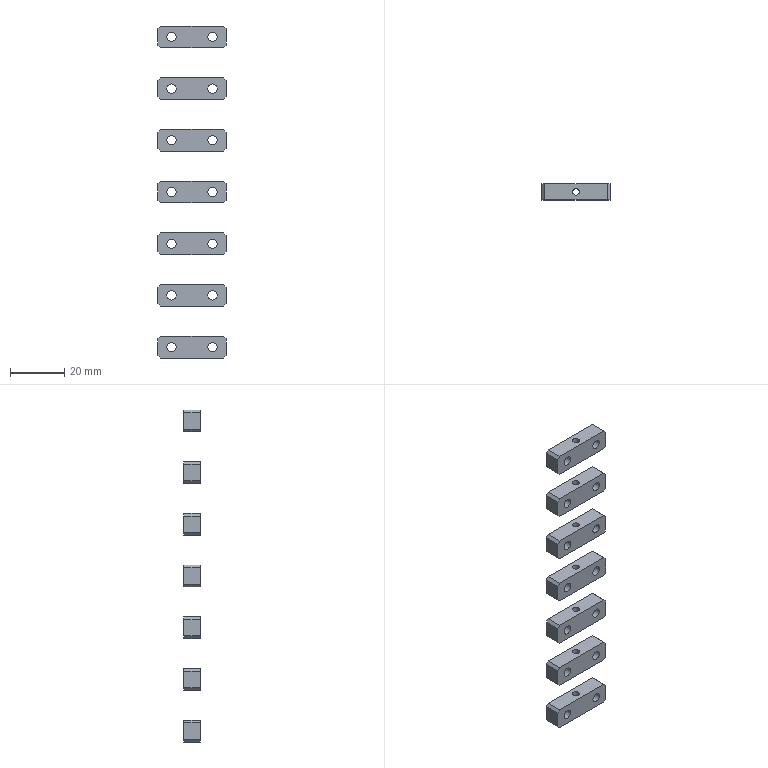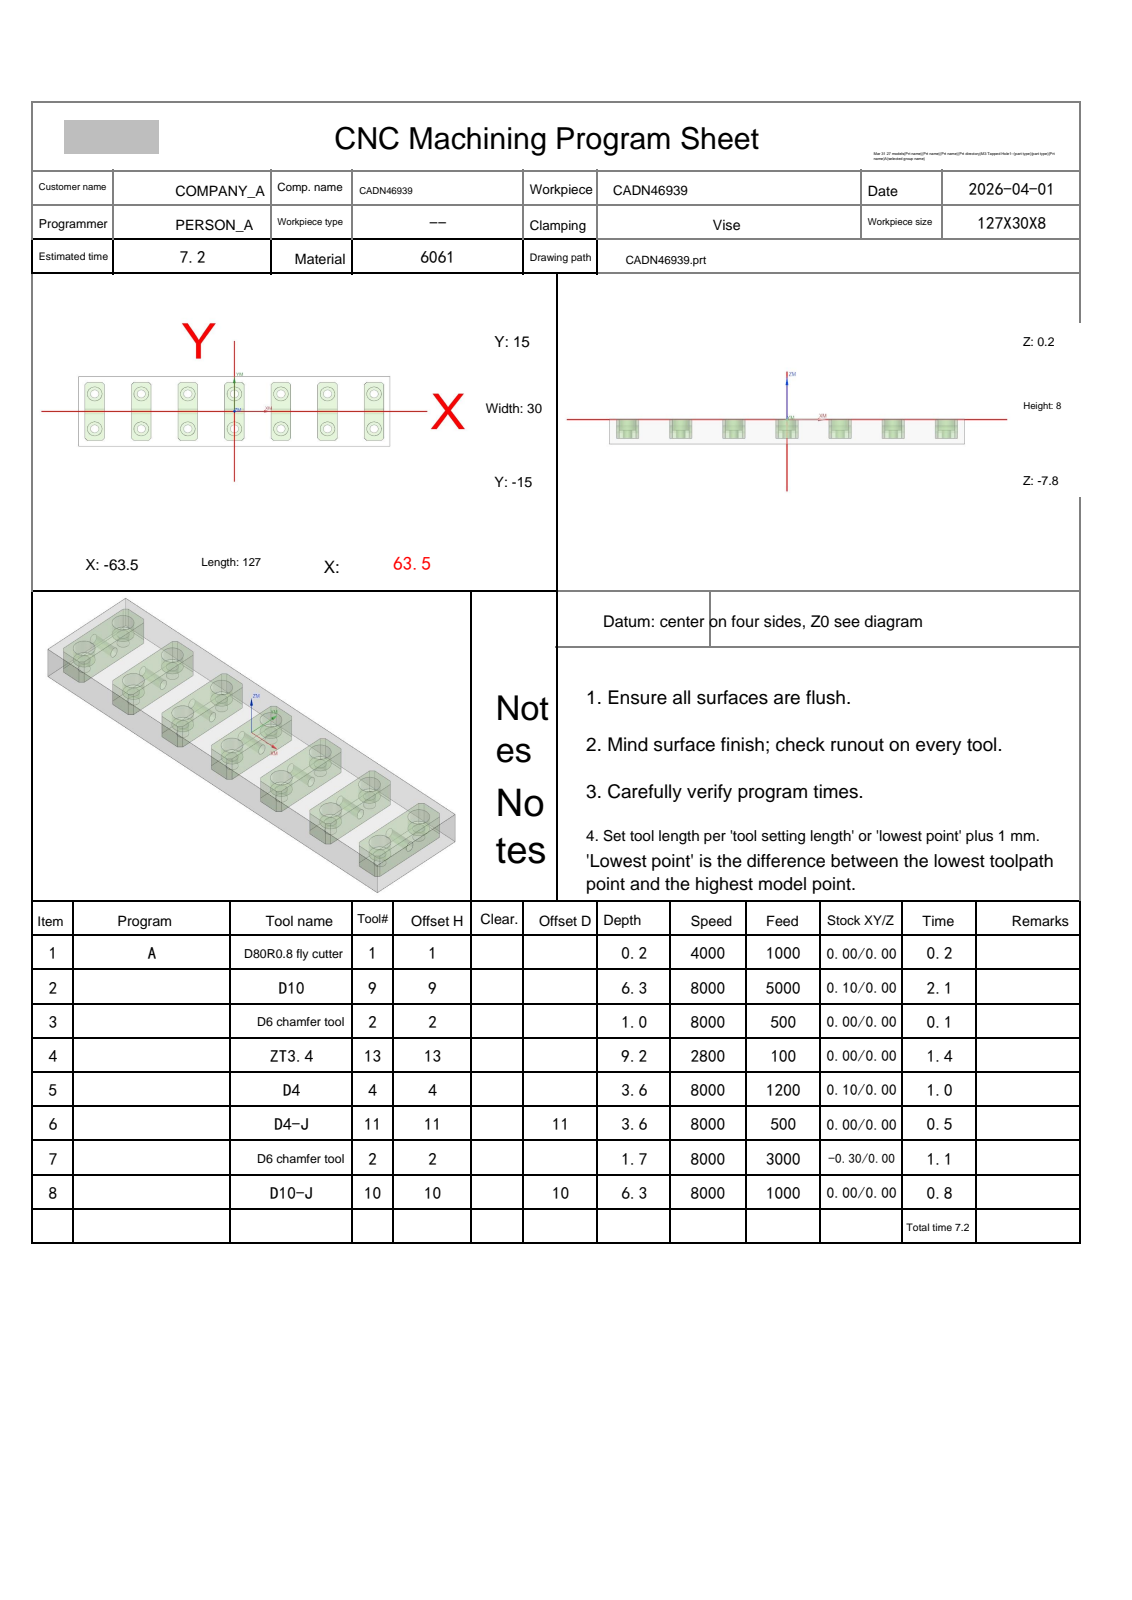NC program | NX | posted by the shop | part box 25 x 6 x 122 mm
Lines 34 to 849 of 3537:
N2 T09 M06
(D10  D=10. R=0. H=09 ce=0.10 di=0.00)
G00 G90 G54 X47.1 Y0.0 M03 S8000
G43 H09 Z20.
M08
Z.5
G01 Y-11.5 Z.443 F5000.
G02 X45.606 Y-15.106 Z.424 I-5.1 J0.0
G01 X44.606 Y-16.106 Z.417
G02 X41. Y-17.6 Z.397 I-3.606 J3.606
G01 X35. Z.367
G02 X31.394 Y-16.106 Z.348 I0.0 J5.1
G01 X30.394 Y-15.106 Z.341
G02 X28.9 Y-11.5 Z.321 I3.606 J3.606
G01 Y11.5 Z.208
G02 X30.394 Y15.106 Z.188 I5.1 J0.0
G01 X31.394 Y16.106 Z.181
G02 X35. Y17.6 Z.161 I3.606 J-3.606
G01 X41. Z.132
G02 X44.606 Y16.106 Z.112 I0.0 J-5.1
G01 X45.606 Y15.106 Z.105
G02 X47.1 Y11.5 Z.085 I-3.606 J-3.606
G01 Y-11.5 Z-.028
G02 X45.606 Y-15.106 Z-.048 I-5.1 J0.0
G01 X44.606 Y-16.106 Z-.055
G02 X41. Y-17.6 Z-.075 I-3.606 J3.606
G01 X35. Z-.104
G02 X31.394 Y-16.106 Z-.124 I0.0 J5.1
G01 X30.394 Y-15.106 Z-.131
G02 X28.9 Y-11.5 Z-.15 I3.606 J3.606
G01 Y11.5 Z-.264
G02 X30.394 Y15.106 Z-.284 I5.1 J0.0
G01 X31.394 Y16.106 Z-.29
G02 X35. Y17.6 Z-.31 I3.606 J-3.606
G01 X41. Z-.34
G02 X44.606 Y16.106 Z-.36 I0.0 J-5.1
G01 X45.606 Y15.106 Z-.366
G02 X47.1 Y11.5 Z-.386 I-3.606 J-3.606
G01 Y-11.5 Z-.5
G02 X45.606 Y-15.106 Z-.519 I-5.1 J0.0
G01 X44.606 Y-16.106 Z-.526
G02 X41. Y-17.6 Z-.546 I-3.606 J3.606
G01 X35. Z-.575
G02 X31.394 Y-16.106 Z-.595 I0.0 J5.1
G01 X30.394 Y-15.106 Z-.602
G02 X28.9 Y-11.5 Z-.622 I3.606 J3.606
G01 Y11.5 Z-.735
G02 X30.394 Y15.106 Z-.755 I5.1 J0.0
G01 X31.394 Y16.106 Z-.762
G02 X35. Y17.6 Z-.782 I3.606 J-3.606
G01 X41. Z-.811
G02 X44.606 Y16.106 Z-.831 I0.0 J-5.1
G01 X45.606 Y15.106 Z-.838
G02 X47.1 Y11.5 Z-.858 I-3.606 J-3.606
G01 Y-11.5 Z-.971
G02 X45.606 Y-15.106 Z-.991 I-5.1 J0.0
G01 X44.606 Y-16.106 Z-.998
G02 X41. Y-17.6 Z-1.017 I-3.606 J3.606
G01 X35. Z-1.047
G02 X31.394 Y-16.106 Z-1.067 I0.0 J5.1
G01 X30.394 Y-15.106 Z-1.074
G02 X28.9 Y-11.5 Z-1.093 I3.606 J3.606
G01 Y11.5 Z-1.207
G02 X30.394 Y15.106 Z-1.226 I5.1 J0.0
G01 X31.394 Y16.106 Z-1.233
G02 X35. Y17.6 Z-1.253 I3.606 J-3.606
G01 X41. Z-1.283
G02 X44.606 Y16.106 Z-1.302 I0.0 J-5.1
G01 X45.606 Y15.106 Z-1.309
G02 X47.1 Y11.5 Z-1.329 I-3.606 J-3.606
G01 Y-11.5 Z-1.442
G02 X45.606 Y-15.106 Z-1.462 I-5.1 J0.0
G01 X44.606 Y-16.106 Z-1.469
G02 X41. Y-17.6 Z-1.489 I-3.606 J3.606
G01 X35. Z-1.518
G02 X31.394 Y-16.106 Z-1.538 I0.0 J5.1
G01 X30.394 Y-15.106 Z-1.545
G02 X28.9 Y-11.5 Z-1.565 I3.606 J3.606
G01 Y11.5 Z-1.678
G02 X30.394 Y15.106 Z-1.698 I5.1 J0.0
G01 X31.394 Y16.106 Z-1.705
G02 X35. Y17.6 Z-1.725 I3.606 J-3.606
G01 X41. Z-1.754
G02 X44.606 Y16.106 Z-1.774 I0.0 J-5.1
G01 X45.606 Y15.106 Z-1.781
G02 X47.1 Y11.5 Z-1.8 I-3.606 J-3.606
G01 Y-11.5 Z-1.914
G02 X45.606 Y-15.106 Z-1.934 I-5.1 J0.0
G01 X44.606 Y-16.106 Z-1.94
G02 X41. Y-17.6 Z-1.96 I-3.606 J3.606
G01 X35. Z-1.99
G02 X31.394 Y-16.106 Z-2.01 I0.0 J5.1
G01 X30.394 Y-15.106 Z-2.016
G02 X28.9 Y-11.5 Z-2.036 I3.606 J3.606
G01 Y11.5 Z-2.15
G02 X30.394 Y15.106 Z-2.169 I5.1 J0.0
G01 X31.394 Y16.106 Z-2.176
G02 X35. Y17.6 Z-2.196 I3.606 J-3.606
G01 X41. Z-2.225
G02 X44.606 Y16.106 Z-2.245 I0.0 J-5.1
G01 X45.606 Y15.106 Z-2.252
G02 X47.1 Y11.5 Z-2.272 I-3.606 J-3.606
G01 Y-11.5 Z-2.385
G02 X45.606 Y-15.106 Z-2.405 I-5.1 J0.0
G01 X44.606 Y-16.106 Z-2.412
G02 X41. Y-17.6 Z-2.432 I-3.606 J3.606
G01 X35. Z-2.461
G02 X31.394 Y-16.106 Z-2.481 I0.0 J5.1
G01 X30.394 Y-15.106 Z-2.488
G02 X28.9 Y-11.5 Z-2.508 I3.606 J3.606
G01 Y11.5 Z-2.621
G02 X30.394 Y15.106 Z-2.641 I5.1 J0.0
G01 X31.394 Y16.106 Z-2.648
G02 X35. Y17.6 Z-2.667 I3.606 J-3.606
G01 X41. Z-2.697
G02 X44.606 Y16.106 Z-2.717 I0.0 J-5.1
G01 X45.606 Y15.106 Z-2.724
G02 X47.1 Y11.5 Z-2.743 I-3.606 J-3.606
G01 Y-11.5 Z-2.857
G02 X45.606 Y-15.106 Z-2.876 I-5.1 J0.0
G01 X44.606 Y-16.106 Z-2.883
G02 X41. Y-17.6 Z-2.903 I-3.606 J3.606
G01 X35. Z-2.933
G02 X31.394 Y-16.106 Z-2.952 I0.0 J5.1
G01 X30.394 Y-15.106 Z-2.959
G02 X28.9 Y-11.5 Z-2.979 I3.606 J3.606
G01 Y11.5 Z-3.092
G02 X30.394 Y15.106 Z-3.112 I5.1 J0.0
G01 X31.394 Y16.106 Z-3.119
G02 X35. Y17.6 Z-3.139 I3.606 J-3.606
G01 X41. Z-3.168
G02 X44.606 Y16.106 Z-3.188 I0.0 J-5.1
G01 X45.606 Y15.106 Z-3.195
G02 X47.1 Y11.5 Z-3.215 I-3.606 J-3.606
G01 Y-11.5 Z-3.328
G02 X45.606 Y-15.106 Z-3.348 I-5.1 J0.0
G01 X44.606 Y-16.106 Z-3.355
G02 X41. Y-17.6 Z-3.375 I-3.606 J3.606
G01 X35. Z-3.404
G02 X31.394 Y-16.106 Z-3.424 I0.0 J5.1
G01 X30.394 Y-15.106 Z-3.431
G02 X28.9 Y-11.5 Z-3.45 I3.606 J3.606
G01 Y11.5 Z-3.564
G02 X30.394 Y15.106 Z-3.584 I5.1 J0.0
G01 X31.394 Y16.106 Z-3.59
G02 X35. Y17.6 Z-3.61 I3.606 J-3.606
G01 X41. Z-3.64
G02 X44.606 Y16.106 Z-3.66 I0.0 J-5.1
G01 X45.606 Y15.106 Z-3.666
G02 X47.1 Y11.5 Z-3.686 I-3.606 J-3.606
G01 Y-11.5 Z-3.8
G02 X45.606 Y-15.106 Z-3.819 I-5.1 J0.0
G01 X44.606 Y-16.106 Z-3.826
G02 X41. Y-17.6 Z-3.846 I-3.606 J3.606
G01 X35. Z-3.875
G02 X31.394 Y-16.106 Z-3.895 I0.0 J5.1
G01 X30.394 Y-15.106 Z-3.902
G02 X28.9 Y-11.5 Z-3.922 I3.606 J3.606
G01 Y11.5 Z-4.035
G02 X30.394 Y15.106 Z-4.055 I5.1 J0.0
G01 X31.394 Y16.106 Z-4.062
G02 X35. Y17.6 Z-4.082 I3.606 J-3.606
G01 X41. Z-4.111
G02 X44.606 Y16.106 Z-4.131 I0.0 J-5.1
G01 X45.606 Y15.106 Z-4.138
G02 X47.1 Y11.5 Z-4.158 I-3.606 J-3.606
G01 Y-11.5 Z-4.271
G02 X45.606 Y-15.106 Z-4.291 I-5.1 J0.0
G01 X44.606 Y-16.106 Z-4.298
G02 X41. Y-17.6 Z-4.317 I-3.606 J3.606
G01 X35. Z-4.347
G02 X31.394 Y-16.106 Z-4.367 I0.0 J5.1
G01 X30.394 Y-15.106 Z-4.374
G02 X28.9 Y-11.5 Z-4.393 I3.606 J3.606
G01 Y11.5 Z-4.507
G02 X30.394 Y15.106 Z-4.526 I5.1 J0.0
G01 X31.394 Y16.106 Z-4.533
G02 X35. Y17.6 Z-4.553 I3.606 J-3.606
G01 X41. Z-4.583
G02 X44.606 Y16.106 Z-4.602 I0.0 J-5.1
G01 X45.606 Y15.106 Z-4.609
G02 X47.1 Y11.5 Z-4.629 I-3.606 J-3.606
G01 Y-11.5 Z-4.742
G02 X45.606 Y-15.106 Z-4.762 I-5.1 J0.0
G01 X44.606 Y-16.106 Z-4.769
G02 X41. Y-17.6 Z-4.789 I-3.606 J3.606
G01 X35. Z-4.818
G02 X31.394 Y-16.106 Z-4.838 I0.0 J5.1
G01 X30.394 Y-15.106 Z-4.845
G02 X28.9 Y-11.5 Z-4.865 I3.606 J3.606
G01 Y11.5 Z-4.978
G02 X30.394 Y15.106 Z-4.998 I5.1 J0.0
G01 X31.394 Y16.106 Z-5.005
G02 X35. Y17.6 Z-5.025 I3.606 J-3.606
G01 X41. Z-5.054
G02 X44.606 Y16.106 Z-5.074 I0.0 J-5.1
G01 X45.606 Y15.106 Z-5.081
G02 X47.1 Y11.5 Z-5.1 I-3.606 J-3.606
G01 Y-11.5 Z-5.214
G02 X45.606 Y-15.106 Z-5.234 I-5.1 J0.0
G01 X44.606 Y-16.106 Z-5.24
G02 X41. Y-17.6 Z-5.26 I-3.606 J3.606
G01 X35. Z-5.29
G02 X31.394 Y-16.106 Z-5.31 I0.0 J5.1
G01 X30.394 Y-15.106 Z-5.316
G02 X28.9 Y-11.5 Z-5.336 I3.606 J3.606
G01 Y11.5 Z-5.45
G02 X30.394 Y15.106 Z-5.469 I5.1 J0.0
G01 X31.394 Y16.106 Z-5.476
G02 X35. Y17.6 Z-5.496 I3.606 J-3.606
G01 X41. Z-5.525
G02 X44.606 Y16.106 Z-5.545 I0.0 J-5.1
G01 X45.606 Y15.106 Z-5.552
G02 X47.1 Y11.5 Z-5.572 I-3.606 J-3.606
G01 Y-11.5 Z-5.685
G02 X45.606 Y-15.106 Z-5.705 I-5.1 J0.0
G01 X44.606 Y-16.106 Z-5.712
G02 X41. Y-17.6 Z-5.732 I-3.606 J3.606
G01 X35. Z-5.761
G02 X31.394 Y-16.106 Z-5.781 I0.0 J5.1
G01 X30.394 Y-15.106 Z-5.788
G02 X28.9 Y-11.5 Z-5.808 I3.606 J3.606
G01 Y11.5 Z-5.921
G02 X30.394 Y15.106 Z-5.941 I5.1 J0.0
G01 X31.394 Y16.106 Z-5.948
G02 X35. Y17.6 Z-5.967 I3.606 J-3.606
G01 X41. Z-5.997
G02 X44.606 Y16.106 Z-6.017 I0.0 J-5.1
G01 X45.606 Y15.106 Z-6.024
G02 X47.1 Y11.5 Z-6.043 I-3.606 J-3.606
G01 Y0.0 Z-6.1
Y-11.5
G02 X45.606 Y-15.106 I-5.1 J0.0
G01 X44.606 Y-16.106
G02 X41. Y-17.6 I-3.606 J3.606
G01 X35.
G02 X31.394 Y-16.106 I0.0 J5.1
G01 X30.394 Y-15.106
G02 X28.9 Y-11.5 I3.606 J3.606
G01 Y11.5
G02 X30.394 Y15.106 I5.1 J0.0
G01 X31.394 Y16.106
G02 X35. Y17.6 I3.606 J-3.606
G01 X41.
G02 X44.606 Y16.106 I0.0 J-5.1
G01 X45.606 Y15.106
G02 X47.1 Y11.5 I-3.606 J-3.606
G01 Y0.0
Y-.5
Z-5.1
G00 Z20.
X66.1 Y0.0
Z.5
G01 Y-11.5 Z.443
G02 X64.606 Y-15.106 Z.424 I-5.1 J0.0
G01 X63.606 Y-16.106 Z.417
G02 X60. Y-17.6 Z.397 I-3.606 J3.606
G01 X54. Z.367
G02 X50.394 Y-16.106 Z.348 I0.0 J5.1
G01 X49.394 Y-15.106 Z.341
G02 X47.9 Y-11.5 Z.321 I3.606 J3.606
G01 Y11.5 Z.208
G02 X49.394 Y15.106 Z.188 I5.1 J0.0
G01 X50.394 Y16.106 Z.181
G02 X54. Y17.6 Z.161 I3.606 J-3.606
G01 X60. Z.132
G02 X63.606 Y16.106 Z.112 I0.0 J-5.1
G01 X64.606 Y15.106 Z.105
G02 X66.1 Y11.5 Z.085 I-3.606 J-3.606
G01 Y-11.5 Z-.028
G02 X64.606 Y-15.106 Z-.048 I-5.1 J0.0
G01 X63.606 Y-16.106 Z-.055
G02 X60. Y-17.6 Z-.075 I-3.606 J3.606
G01 X54. Z-.104
G02 X50.394 Y-16.106 Z-.124 I0.0 J5.1
G01 X49.394 Y-15.106 Z-.131
G02 X47.9 Y-11.5 Z-.15 I3.606 J3.606
G01 Y11.5 Z-.264
G02 X49.394 Y15.106 Z-.284 I5.1 J0.0
G01 X50.394 Y16.106 Z-.29
G02 X54. Y17.6 Z-.31 I3.606 J-3.606
G01 X60. Z-.34
G02 X63.606 Y16.106 Z-.36 I0.0 J-5.1
G01 X64.606 Y15.106 Z-.366
G02 X66.1 Y11.5 Z-.386 I-3.606 J-3.606
G01 Y-11.5 Z-.5
G02 X64.606 Y-15.106 Z-.519 I-5.1 J0.0
G01 X63.606 Y-16.106 Z-.526
G02 X60. Y-17.6 Z-.546 I-3.606 J3.606
G01 X54. Z-.575
G02 X50.394 Y-16.106 Z-.595 I0.0 J5.1
G01 X49.394 Y-15.106 Z-.602
G02 X47.9 Y-11.5 Z-.622 I3.606 J3.606
G01 Y11.5 Z-.735
G02 X49.394 Y15.106 Z-.755 I5.1 J0.0
G01 X50.394 Y16.106 Z-.762
G02 X54. Y17.6 Z-.782 I3.606 J-3.606
G01 X60. Z-.811
G02 X63.606 Y16.106 Z-.831 I0.0 J-5.1
G01 X64.606 Y15.106 Z-.838
G02 X66.1 Y11.5 Z-.858 I-3.606 J-3.606
G01 Y-11.5 Z-.971
G02 X64.606 Y-15.106 Z-.991 I-5.1 J0.0
G01 X63.606 Y-16.106 Z-.998
G02 X60. Y-17.6 Z-1.017 I-3.606 J3.606
G01 X54. Z-1.047
G02 X50.394 Y-16.106 Z-1.067 I0.0 J5.1
G01 X49.394 Y-15.106 Z-1.074
G02 X47.9 Y-11.5 Z-1.093 I3.606 J3.606
G01 Y11.5 Z-1.207
G02 X49.394 Y15.106 Z-1.226 I5.1 J0.0
G01 X50.394 Y16.106 Z-1.233
G02 X54. Y17.6 Z-1.253 I3.606 J-3.606
G01 X60. Z-1.283
G02 X63.606 Y16.106 Z-1.302 I0.0 J-5.1
G01 X64.606 Y15.106 Z-1.309
G02 X66.1 Y11.5 Z-1.329 I-3.606 J-3.606
G01 Y-11.5 Z-1.442
G02 X64.606 Y-15.106 Z-1.462 I-5.1 J0.0
G01 X63.606 Y-16.106 Z-1.469
G02 X60. Y-17.6 Z-1.489 I-3.606 J3.606
G01 X54. Z-1.518
G02 X50.394 Y-16.106 Z-1.538 I0.0 J5.1
G01 X49.394 Y-15.106 Z-1.545
G02 X47.9 Y-11.5 Z-1.565 I3.606 J3.606
G01 Y11.5 Z-1.678
G02 X49.394 Y15.106 Z-1.698 I5.1 J0.0
G01 X50.394 Y16.106 Z-1.705
G02 X54. Y17.6 Z-1.725 I3.606 J-3.606
G01 X60. Z-1.754
G02 X63.606 Y16.106 Z-1.774 I0.0 J-5.1
G01 X64.606 Y15.106 Z-1.781
G02 X66.1 Y11.5 Z-1.8 I-3.606 J-3.606
G01 Y-11.5 Z-1.914
G02 X64.606 Y-15.106 Z-1.934 I-5.1 J0.0
G01 X63.606 Y-16.106 Z-1.94
G02 X60. Y-17.6 Z-1.96 I-3.606 J3.606
G01 X54. Z-1.99
G02 X50.394 Y-16.106 Z-2.01 I0.0 J5.1
G01 X49.394 Y-15.106 Z-2.016
G02 X47.9 Y-11.5 Z-2.036 I3.606 J3.606
G01 Y11.5 Z-2.15
G02 X49.394 Y15.106 Z-2.169 I5.1 J0.0
G01 X50.394 Y16.106 Z-2.176
G02 X54. Y17.6 Z-2.196 I3.606 J-3.606
G01 X60. Z-2.225
G02 X63.606 Y16.106 Z-2.245 I0.0 J-5.1
G01 X64.606 Y15.106 Z-2.252
G02 X66.1 Y11.5 Z-2.272 I-3.606 J-3.606
G01 Y-11.5 Z-2.385
G02 X64.606 Y-15.106 Z-2.405 I-5.1 J0.0
G01 X63.606 Y-16.106 Z-2.412
G02 X60. Y-17.6 Z-2.432 I-3.606 J3.606
G01 X54. Z-2.461
G02 X50.394 Y-16.106 Z-2.481 I0.0 J5.1
G01 X49.394 Y-15.106 Z-2.488
G02 X47.9 Y-11.5 Z-2.508 I3.606 J3.606
G01 Y11.5 Z-2.621
G02 X49.394 Y15.106 Z-2.641 I5.1 J0.0
G01 X50.394 Y16.106 Z-2.648
G02 X54. Y17.6 Z-2.667 I3.606 J-3.606
G01 X60. Z-2.697
G02 X63.606 Y16.106 Z-2.717 I0.0 J-5.1
G01 X64.606 Y15.106 Z-2.724
G02 X66.1 Y11.5 Z-2.743 I-3.606 J-3.606
G01 Y-11.5 Z-2.857
G02 X64.606 Y-15.106 Z-2.876 I-5.1 J0.0
G01 X63.606 Y-16.106 Z-2.883
G02 X60. Y-17.6 Z-2.903 I-3.606 J3.606
G01 X54. Z-2.933
G02 X50.394 Y-16.106 Z-2.952 I0.0 J5.1
G01 X49.394 Y-15.106 Z-2.959
G02 X47.9 Y-11.5 Z-2.979 I3.606 J3.606
G01 Y11.5 Z-3.092
G02 X49.394 Y15.106 Z-3.112 I5.1 J0.0
G01 X50.394 Y16.106 Z-3.119
G02 X54. Y17.6 Z-3.139 I3.606 J-3.606
G01 X60. Z-3.168
G02 X63.606 Y16.106 Z-3.188 I0.0 J-5.1
G01 X64.606 Y15.106 Z-3.195
G02 X66.1 Y11.5 Z-3.215 I-3.606 J-3.606
G01 Y-11.5 Z-3.328
G02 X64.606 Y-15.106 Z-3.348 I-5.1 J0.0
G01 X63.606 Y-16.106 Z-3.355
G02 X60. Y-17.6 Z-3.375 I-3.606 J3.606
G01 X54. Z-3.404
G02 X50.394 Y-16.106 Z-3.424 I0.0 J5.1
G01 X49.394 Y-15.106 Z-3.431
G02 X47.9 Y-11.5 Z-3.45 I3.606 J3.606
G01 Y11.5 Z-3.564
G02 X49.394 Y15.106 Z-3.584 I5.1 J0.0
G01 X50.394 Y16.106 Z-3.59
G02 X54. Y17.6 Z-3.61 I3.606 J-3.606
G01 X60. Z-3.64
G02 X63.606 Y16.106 Z-3.66 I0.0 J-5.1
G01 X64.606 Y15.106 Z-3.666
G02 X66.1 Y11.5 Z-3.686 I-3.606 J-3.606
G01 Y-11.5 Z-3.8
G02 X64.606 Y-15.106 Z-3.819 I-5.1 J0.0
G01 X63.606 Y-16.106 Z-3.826
G02 X60. Y-17.6 Z-3.846 I-3.606 J3.606
G01 X54. Z-3.875
G02 X50.394 Y-16.106 Z-3.895 I0.0 J5.1
G01 X49.394 Y-15.106 Z-3.902
G02 X47.9 Y-11.5 Z-3.922 I3.606 J3.606
G01 Y11.5 Z-4.035
G02 X49.394 Y15.106 Z-4.055 I5.1 J0.0
G01 X50.394 Y16.106 Z-4.062
G02 X54. Y17.6 Z-4.082 I3.606 J-3.606
G01 X60. Z-4.111
G02 X63.606 Y16.106 Z-4.131 I0.0 J-5.1
G01 X64.606 Y15.106 Z-4.138
G02 X66.1 Y11.5 Z-4.158 I-3.606 J-3.606
G01 Y-11.5 Z-4.271
G02 X64.606 Y-15.106 Z-4.291 I-5.1 J0.0
G01 X63.606 Y-16.106 Z-4.298
G02 X60. Y-17.6 Z-4.317 I-3.606 J3.606
G01 X54. Z-4.347
G02 X50.394 Y-16.106 Z-4.367 I0.0 J5.1
G01 X49.394 Y-15.106 Z-4.374
G02 X47.9 Y-11.5 Z-4.393 I3.606 J3.606
G01 Y11.5 Z-4.507
G02 X49.394 Y15.106 Z-4.526 I5.1 J0.0
G01 X50.394 Y16.106 Z-4.533
G02 X54. Y17.6 Z-4.553 I3.606 J-3.606
G01 X60. Z-4.583
G02 X63.606 Y16.106 Z-4.602 I0.0 J-5.1
G01 X64.606 Y15.106 Z-4.609
G02 X66.1 Y11.5 Z-4.629 I-3.606 J-3.606
G01 Y-11.5 Z-4.742
G02 X64.606 Y-15.106 Z-4.762 I-5.1 J0.0
G01 X63.606 Y-16.106 Z-4.769
G02 X60. Y-17.6 Z-4.789 I-3.606 J3.606
G01 X54. Z-4.818
G02 X50.394 Y-16.106 Z-4.838 I0.0 J5.1
G01 X49.394 Y-15.106 Z-4.845
G02 X47.9 Y-11.5 Z-4.865 I3.606 J3.606
G01 Y11.5 Z-4.978
G02 X49.394 Y15.106 Z-4.998 I5.1 J0.0
G01 X50.394 Y16.106 Z-5.005
G02 X54. Y17.6 Z-5.025 I3.606 J-3.606
G01 X60. Z-5.054
G02 X63.606 Y16.106 Z-5.074 I0.0 J-5.1
G01 X64.606 Y15.106 Z-5.081
G02 X66.1 Y11.5 Z-5.1 I-3.606 J-3.606
G01 Y-11.5 Z-5.214
G02 X64.606 Y-15.106 Z-5.234 I-5.1 J0.0
G01 X63.606 Y-16.106 Z-5.24
G02 X60. Y-17.6 Z-5.26 I-3.606 J3.606
G01 X54. Z-5.29
G02 X50.394 Y-16.106 Z-5.31 I0.0 J5.1
G01 X49.394 Y-15.106 Z-5.316
G02 X47.9 Y-11.5 Z-5.336 I3.606 J3.606
G01 Y11.5 Z-5.45
G02 X49.394 Y15.106 Z-5.469 I5.1 J0.0
G01 X50.394 Y16.106 Z-5.476
G02 X54. Y17.6 Z-5.496 I3.606 J-3.606
G01 X60. Z-5.525
G02 X63.606 Y16.106 Z-5.545 I0.0 J-5.1
G01 X64.606 Y15.106 Z-5.552
G02 X66.1 Y11.5 Z-5.572 I-3.606 J-3.606
G01 Y-11.5 Z-5.685
G02 X64.606 Y-15.106 Z-5.705 I-5.1 J0.0
G01 X63.606 Y-16.106 Z-5.712
G02 X60. Y-17.6 Z-5.732 I-3.606 J3.606
G01 X54. Z-5.761
G02 X50.394 Y-16.106 Z-5.781 I0.0 J5.1
G01 X49.394 Y-15.106 Z-5.788
G02 X47.9 Y-11.5 Z-5.808 I3.606 J3.606
G01 Y11.5 Z-5.921
G02 X49.394 Y15.106 Z-5.941 I5.1 J0.0
G01 X50.394 Y16.106 Z-5.948
G02 X54. Y17.6 Z-5.967 I3.606 J-3.606
G01 X60. Z-5.997
G02 X63.606 Y16.106 Z-6.017 I0.0 J-5.1
G01 X64.606 Y15.106 Z-6.024
G02 X66.1 Y11.5 Z-6.043 I-3.606 J-3.606
G01 Y0.0 Z-6.1
Y-11.5
G02 X64.606 Y-15.106 I-5.1 J0.0
G01 X63.606 Y-16.106
G02 X60. Y-17.6 I-3.606 J3.606
G01 X54.
G02 X50.394 Y-16.106 I0.0 J5.1
G01 X49.394 Y-15.106
G02 X47.9 Y-11.5 I3.606 J3.606
G01 Y11.5
G02 X49.394 Y15.106 I5.1 J0.0
G01 X50.394 Y16.106
G02 X54. Y17.6 I3.606 J-3.606
G01 X60.
G02 X63.606 Y16.106 I0.0 J-5.1
G01 X64.606 Y15.106
G02 X66.1 Y11.5 I-3.606 J-3.606
G01 Y0.0
Y-.5
Z-5.1
G00 Z20.
X28.1 Y0.0
Z.5
G01 Y-11.5 Z.443
G02 X26.606 Y-15.106 Z.424 I-5.1 J0.0
G01 X25.606 Y-16.106 Z.417
G02 X22. Y-17.6 Z.397 I-3.606 J3.606
G01 X16. Z.367
G02 X12.394 Y-16.106 Z.348 I0.0 J5.1
G01 X11.394 Y-15.106 Z.341
G02 X9.9 Y-11.5 Z.321 I3.606 J3.606
G01 Y11.5 Z.208
G02 X11.394 Y15.106 Z.188 I5.1 J0.0
G01 X12.394 Y16.106 Z.181
G02 X16. Y17.6 Z.161 I3.606 J-3.606
G01 X22. Z.132
G02 X25.606 Y16.106 Z.112 I0.0 J-5.1
G01 X26.606 Y15.106 Z.105
G02 X28.1 Y11.5 Z.085 I-3.606 J-3.606
G01 Y-11.5 Z-.028
G02 X26.606 Y-15.106 Z-.048 I-5.1 J0.0
G01 X25.606 Y-16.106 Z-.055
G02 X22. Y-17.6 Z-.075 I-3.606 J3.606
G01 X16. Z-.104
G02 X12.394 Y-16.106 Z-.124 I0.0 J5.1
G01 X11.394 Y-15.106 Z-.131
G02 X9.9 Y-11.5 Z-.15 I3.606 J3.606
G01 Y11.5 Z-.264
G02 X11.394 Y15.106 Z-.284 I5.1 J0.0
G01 X12.394 Y16.106 Z-.29
G02 X16. Y17.6 Z-.31 I3.606 J-3.606
G01 X22. Z-.34
G02 X25.606 Y16.106 Z-.36 I0.0 J-5.1
G01 X26.606 Y15.106 Z-.366
G02 X28.1 Y11.5 Z-.386 I-3.606 J-3.606
G01 Y-11.5 Z-.5
G02 X26.606 Y-15.106 Z-.519 I-5.1 J0.0
G01 X25.606 Y-16.106 Z-.526
G02 X22. Y-17.6 Z-.546 I-3.606 J3.606
G01 X16. Z-.575
G02 X12.394 Y-16.106 Z-.595 I0.0 J5.1
G01 X11.394 Y-15.106 Z-.602
G02 X9.9 Y-11.5 Z-.622 I3.606 J3.606
G01 Y11.5 Z-.735
G02 X11.394 Y15.106 Z-.755 I5.1 J0.0
G01 X12.394 Y16.106 Z-.762
G02 X16. Y17.6 Z-.782 I3.606 J-3.606
G01 X22. Z-.811
G02 X25.606 Y16.106 Z-.831 I0.0 J-5.1
G01 X26.606 Y15.106 Z-.838
G02 X28.1 Y11.5 Z-.858 I-3.606 J-3.606
G01 Y-11.5 Z-.971
G02 X26.606 Y-15.106 Z-.991 I-5.1 J0.0
G01 X25.606 Y-16.106 Z-.998
G02 X22. Y-17.6 Z-1.017 I-3.606 J3.606
G01 X16. Z-1.047
G02 X12.394 Y-16.106 Z-1.067 I0.0 J5.1
G01 X11.394 Y-15.106 Z-1.074
G02 X9.9 Y-11.5 Z-1.093 I3.606 J3.606
G01 Y11.5 Z-1.207
G02 X11.394 Y15.106 Z-1.226 I5.1 J0.0
G01 X12.394 Y16.106 Z-1.233
G02 X16. Y17.6 Z-1.253 I3.606 J-3.606
G01 X22. Z-1.283
G02 X25.606 Y16.106 Z-1.302 I0.0 J-5.1
G01 X26.606 Y15.106 Z-1.309
G02 X28.1 Y11.5 Z-1.329 I-3.606 J-3.606
G01 Y-11.5 Z-1.442
G02 X26.606 Y-15.106 Z-1.462 I-5.1 J0.0
G01 X25.606 Y-16.106 Z-1.469
G02 X22. Y-17.6 Z-1.489 I-3.606 J3.606
G01 X16. Z-1.518
G02 X12.394 Y-16.106 Z-1.538 I0.0 J5.1
G01 X11.394 Y-15.106 Z-1.545
G02 X9.9 Y-11.5 Z-1.565 I3.606 J3.606
G01 Y11.5 Z-1.678
G02 X11.394 Y15.106 Z-1.698 I5.1 J0.0
G01 X12.394 Y16.106 Z-1.705
G02 X16. Y17.6 Z-1.725 I3.606 J-3.606
G01 X22. Z-1.754
G02 X25.606 Y16.106 Z-1.774 I0.0 J-5.1
G01 X26.606 Y15.106 Z-1.781
G02 X28.1 Y11.5 Z-1.8 I-3.606 J-3.606
G01 Y-11.5 Z-1.914
G02 X26.606 Y-15.106 Z-1.934 I-5.1 J0.0
G01 X25.606 Y-16.106 Z-1.94
G02 X22. Y-17.6 Z-1.96 I-3.606 J3.606
G01 X16. Z-1.99
G02 X12.394 Y-16.106 Z-2.01 I0.0 J5.1
G01 X11.394 Y-15.106 Z-2.016
G02 X9.9 Y-11.5 Z-2.036 I3.606 J3.606
G01 Y11.5 Z-2.15
G02 X11.394 Y15.106 Z-2.169 I5.1 J0.0
G01 X12.394 Y16.106 Z-2.176
G02 X16. Y17.6 Z-2.196 I3.606 J-3.606
G01 X22. Z-2.225
G02 X25.606 Y16.106 Z-2.245 I0.0 J-5.1
G01 X26.606 Y15.106 Z-2.252
G02 X28.1 Y11.5 Z-2.272 I-3.606 J-3.606
G01 Y-11.5 Z-2.385
G02 X26.606 Y-15.106 Z-2.405 I-5.1 J0.0
G01 X25.606 Y-16.106 Z-2.412
G02 X22. Y-17.6 Z-2.432 I-3.606 J3.606
G01 X16. Z-2.461
G02 X12.394 Y-16.106 Z-2.481 I0.0 J5.1
G01 X11.394 Y-15.106 Z-2.488
G02 X9.9 Y-11.5 Z-2.508 I3.606 J3.606
G01 Y11.5 Z-2.621
G02 X11.394 Y15.106 Z-2.641 I5.1 J0.0
G01 X12.394 Y16.106 Z-2.648
G02 X16. Y17.6 Z-2.667 I3.606 J-3.606
G01 X22. Z-2.697
G02 X25.606 Y16.106 Z-2.717 I0.0 J-5.1
G01 X26.606 Y15.106 Z-2.724
G02 X28.1 Y11.5 Z-2.743 I-3.606 J-3.606
G01 Y-11.5 Z-2.857
G02 X26.606 Y-15.106 Z-2.876 I-5.1 J0.0
G01 X25.606 Y-16.106 Z-2.883
G02 X22. Y-17.6 Z-2.903 I-3.606 J3.606
G01 X16. Z-2.933
G02 X12.394 Y-16.106 Z-2.952 I0.0 J5.1
G01 X11.394 Y-15.106 Z-2.959
G02 X9.9 Y-11.5 Z-2.979 I3.606 J3.606
G01 Y11.5 Z-3.092
G02 X11.394 Y15.106 Z-3.112 I5.1 J0.0
G01 X12.394 Y16.106 Z-3.119
G02 X16. Y17.6 Z-3.139 I3.606 J-3.606
G01 X22. Z-3.168
G02 X25.606 Y16.106 Z-3.188 I0.0 J-5.1
G01 X26.606 Y15.106 Z-3.195
G02 X28.1 Y11.5 Z-3.215 I-3.606 J-3.606
G01 Y-11.5 Z-3.328
G02 X26.606 Y-15.106 Z-3.348 I-5.1 J0.0
G01 X25.606 Y-16.106 Z-3.355
G02 X22. Y-17.6 Z-3.375 I-3.606 J3.606
G01 X16. Z-3.404
G02 X12.394 Y-16.106 Z-3.424 I0.0 J5.1
G01 X11.394 Y-15.106 Z-3.431
G02 X9.9 Y-11.5 Z-3.45 I3.606 J3.606
G01 Y11.5 Z-3.564
G02 X11.394 Y15.106 Z-3.584 I5.1 J0.0
G01 X12.394 Y16.106 Z-3.59
G02 X16. Y17.6 Z-3.61 I3.606 J-3.606
G01 X22. Z-3.64
G02 X25.606 Y16.106 Z-3.66 I0.0 J-5.1
G01 X26.606 Y15.106 Z-3.666
G02 X28.1 Y11.5 Z-3.686 I-3.606 J-3.606
G01 Y-11.5 Z-3.8
G02 X26.606 Y-15.106 Z-3.819 I-5.1 J0.0
G01 X25.606 Y-16.106 Z-3.826
G02 X22. Y-17.6 Z-3.846 I-3.606 J3.606
G01 X16. Z-3.875
G02 X12.394 Y-16.106 Z-3.895 I0.0 J5.1
G01 X11.394 Y-15.106 Z-3.902
G02 X9.9 Y-11.5 Z-3.922 I3.606 J3.606
G01 Y11.5 Z-4.035
G02 X11.394 Y15.106 Z-4.055 I5.1 J0.0
G01 X12.394 Y16.106 Z-4.062
G02 X16. Y17.6 Z-4.082 I3.606 J-3.606
G01 X22. Z-4.111
G02 X25.606 Y16.106 Z-4.131 I0.0 J-5.1
G01 X26.606 Y15.106 Z-4.138
G02 X28.1 Y11.5 Z-4.158 I-3.606 J-3.606
G01 Y-11.5 Z-4.271
G02 X26.606 Y-15.106 Z-4.291 I-5.1 J0.0
G01 X25.606 Y-16.106 Z-4.298
G02 X22. Y-17.6 Z-4.317 I-3.606 J3.606
G01 X16. Z-4.347
G02 X12.394 Y-16.106 Z-4.367 I0.0 J5.1
G01 X11.394 Y-15.106 Z-4.374
G02 X9.9 Y-11.5 Z-4.393 I3.606 J3.606
G01 Y11.5 Z-4.507
G02 X11.394 Y15.106 Z-4.526 I5.1 J0.0
G01 X12.394 Y16.106 Z-4.533
G02 X16. Y17.6 Z-4.553 I3.606 J-3.606
G01 X22. Z-4.583
G02 X25.606 Y16.106 Z-4.602 I0.0 J-5.1
G01 X26.606 Y15.106 Z-4.609
G02 X28.1 Y11.5 Z-4.629 I-3.606 J-3.606
G01 Y-11.5 Z-4.742
G02 X26.606 Y-15.106 Z-4.762 I-5.1 J0.0
G01 X25.606 Y-16.106 Z-4.769
G02 X22. Y-17.6 Z-4.789 I-3.606 J3.606
G01 X16. Z-4.818
G02 X12.394 Y-16.106 Z-4.838 I0.0 J5.1
G01 X11.394 Y-15.106 Z-4.845
G02 X9.9 Y-11.5 Z-4.865 I3.606 J3.606
G01 Y11.5 Z-4.978
G02 X11.394 Y15.106 Z-4.998 I5.1 J0.0
G01 X12.394 Y16.106 Z-5.005
G02 X16. Y17.6 Z-5.025 I3.606 J-3.606
G01 X22. Z-5.054
G02 X25.606 Y16.106 Z-5.074 I0.0 J-5.1
G01 X26.606 Y15.106 Z-5.081
G02 X28.1 Y11.5 Z-5.1 I-3.606 J-3.606
G01 Y-11.5 Z-5.214
G02 X26.606 Y-15.106 Z-5.234 I-5.1 J0.0
G01 X25.606 Y-16.106 Z-5.24
G02 X22. Y-17.6 Z-5.26 I-3.606 J3.606
G01 X16. Z-5.29
G02 X12.394 Y-16.106 Z-5.31 I0.0 J5.1
G01 X11.394 Y-15.106 Z-5.316
G02 X9.9 Y-11.5 Z-5.336 I3.606 J3.606
G01 Y11.5 Z-5.45
G02 X11.394 Y15.106 Z-5.469 I5.1 J0.0
G01 X12.394 Y16.106 Z-5.476
G02 X16. Y17.6 Z-5.496 I3.606 J-3.606
G01 X22. Z-5.525
G02 X25.606 Y16.106 Z-5.545 I0.0 J-5.1
G01 X26.606 Y15.106 Z-5.552
G02 X28.1 Y11.5 Z-5.572 I-3.606 J-3.606
G01 Y-11.5 Z-5.685
G02 X26.606 Y-15.106 Z-5.705 I-5.1 J0.0
G01 X25.606 Y-16.106 Z-5.712
G02 X22. Y-17.6 Z-5.732 I-3.606 J3.606
G01 X16. Z-5.761
G02 X12.394 Y-16.106 Z-5.781 I0.0 J5.1
G01 X11.394 Y-15.106 Z-5.788
G02 X9.9 Y-11.5 Z-5.808 I3.606 J3.606
G01 Y11.5 Z-5.921
G02 X11.394 Y15.106 Z-5.941 I5.1 J0.0
G01 X12.394 Y16.106 Z-5.948
G02 X16. Y17.6 Z-5.967 I3.606 J-3.606
G01 X22. Z-5.997
G02 X25.606 Y16.106 Z-6.017 I0.0 J-5.1
G01 X26.606 Y15.106 Z-6.024
G02 X28.1 Y11.5 Z-6.043 I-3.606 J-3.606
G01 Y0.0 Z-6.1
Y-11.5
G02 X26.606 Y-15.106 I-5.1 J0.0
G01 X25.606 Y-16.106
G02 X22. Y-17.6 I-3.606 J3.606
G01 X16.
G02 X12.394 Y-16.106 I0.0 J5.1
G01 X11.394 Y-15.106
G02 X9.9 Y-11.5 I3.606 J3.606
G01 Y11.5
G02 X11.394 Y15.106 I5.1 J0.0
G01 X12.394 Y16.106
G02 X16. Y17.6 I3.606 J-3.606
G01 X22.
G02 X25.606 Y16.106 I0.0 J-5.1
G01 X26.606 Y15.106
G02 X28.1 Y11.5 I-3.606 J-3.606
G01 Y0.0
Y-.5
Z-5.1
G00 Z20.
X9.1 Y0.0
Z.5
G01 Y-11.5 Z.443
G02 X7.606 Y-15.106 Z.424 I-5.1 J0.0
G01 X6.606 Y-16.106 Z.417
G02 X3. Y-17.6 Z.397 I-3.606 J3.606
G01 X-3. Z.367
G02 X-6.606 Y-16.106 Z.348 I0.0 J5.1
G01 X-7.606 Y-15.106 Z.341
G02 X-9.1 Y-11.5 Z.321 I3.606 J3.606
G01 Y11.5 Z.208
G02 X-7.606 Y15.106 Z.188 I5.1 J0.0
G01 X-6.606 Y16.106 Z.181
G02 X-3. Y17.6 Z.161 I3.606 J-3.606
G01 X3. Z.132
G02 X6.606 Y16.106 Z.112 I0.0 J-5.1
G01 X7.606 Y15.106 Z.105
G02 X9.1 Y11.5 Z.085 I-3.606 J-3.606
G01 Y-11.5 Z-.028
G02 X7.606 Y-15.106 Z-.048 I-5.1 J0.0
G01 X6.606 Y-16.106 Z-.055
G02 X3. Y-17.6 Z-.075 I-3.606 J3.606
G01 X-3. Z-.104
G02 X-6.606 Y-16.106 Z-.124 I0.0 J5.1
G01 X-7.606 Y-15.106 Z-.131
G02 X-9.1 Y-11.5 Z-.15 I3.606 J3.606
G01 Y11.5 Z-.264
G02 X-7.606 Y15.106 Z-.284 I5.1 J0.0
G01 X-6.606 Y16.106 Z-.29
G02 X-3. Y17.6 Z-.31 I3.606 J-3.606
G01 X3. Z-.34
G02 X6.606 Y16.106 Z-.36 I0.0 J-5.1
G01 X7.606 Y15.106 Z-.366
G02 X9.1 Y11.5 Z-.386 I-3.606 J-3.606
G01 Y-11.5 Z-.5
G02 X7.606 Y-15.106 Z-.519 I-5.1 J0.0
G01 X6.606 Y-16.106 Z-.526
G02 X3. Y-17.6 Z-.546 I-3.606 J3.606
G01 X-3. Z-.575
G02 X-6.606 Y-16.106 Z-.595 I0.0 J5.1
G01 X-7.606 Y-15.106 Z-.602
G02 X-9.1 Y-11.5 Z-.622 I3.606 J3.606
G01 Y11.5 Z-.735
G02 X-7.606 Y15.106 Z-.755 I5.1 J0.0
G01 X-6.606 Y16.106 Z-.762
G02 X-3. Y17.6 Z-.782 I3.606 J-3.606
G01 X3. Z-.811
G02 X6.606 Y16.106 Z-.831 I0.0 J-5.1
G01 X7.606 Y15.106 Z-.838
G02 X9.1 Y11.5 Z-.858 I-3.606 J-3.606
G01 Y-11.5 Z-.971
G02 X7.606 Y-15.106 Z-.991 I-5.1 J0.0
G01 X6.606 Y-16.106 Z-.998
G02 X3. Y-17.6 Z-1.017 I-3.606 J3.606
G01 X-3. Z-1.047
G02 X-6.606 Y-16.106 Z-1.067 I0.0 J5.1
G01 X-7.606 Y-15.106 Z-1.074
G02 X-9.1 Y-11.5 Z-1.093 I3.606 J3.606
G01 Y11.5 Z-1.207
G02 X-7.606 Y15.106 Z-1.226 I5.1 J0.0
G01 X-6.606 Y16.106 Z-1.233
G02 X-3. Y17.6 Z-1.253 I3.606 J-3.606
G01 X3. Z-1.283
G02 X6.606 Y16.106 Z-1.302 I0.0 J-5.1
G01 X7.606 Y15.106 Z-1.309
G02 X9.1 Y11.5 Z-1.329 I-3.606 J-3.606
G01 Y-11.5 Z-1.442
G02 X7.606 Y-15.106 Z-1.462 I-5.1 J0.0
G01 X6.606 Y-16.106 Z-1.469
G02 X3. Y-17.6 Z-1.489 I-3.606 J3.606
G01 X-3. Z-1.518